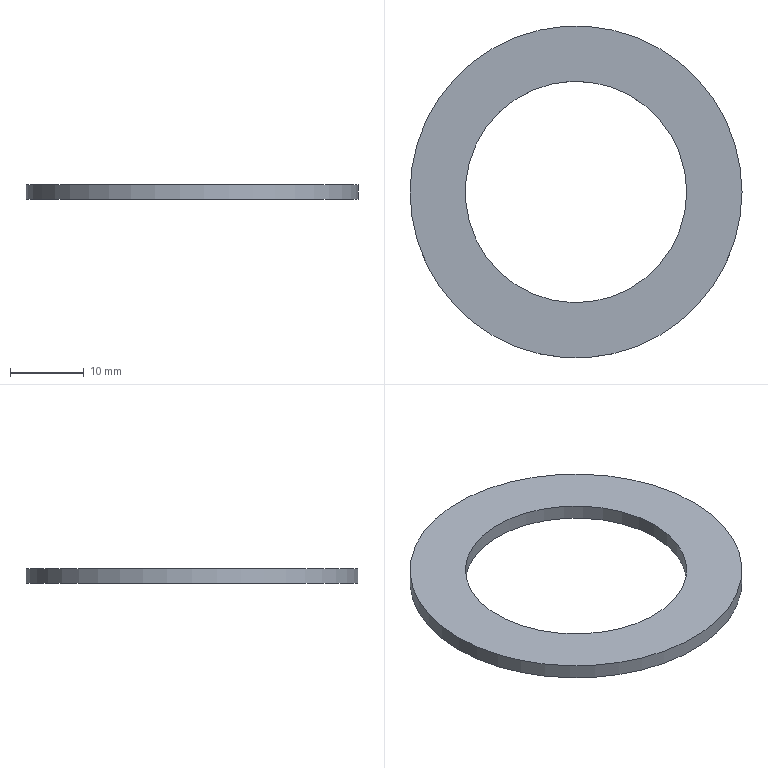Part | NX | features CYLINDER 1, DATUM_CSYS 1, HOLE PACKAGE 1, SIMPLE HOLE 1 | 1 solid | 4 faces | box 45 x 45 x 2 mm | volume 1767 mm3 | plane 2 | cylinder 2 | commonest cylinder face diameters 30 x1 45 x1
STEP:
#1=CARTESIAN_POINT('',(15.,0.,2.));
#2=VERTEX_POINT('',#1);
#3=CARTESIAN_POINT('',(0.,0.,2.));
#4=DIRECTION('',(0.,0.,1.));
#5=DIRECTION('',(1.,0.,0.));
#6=AXIS2_PLACEMENT_3D('',#3,#4,#5);
#7=CIRCLE('',#6,15.);
#8=EDGE_CURVE('',#2,#2,#7,.T.);
#9=ORIENTED_EDGE('',*,*,#8,.F.);
#10=EDGE_LOOP('',(#9));
#11=FACE_BOUND('',#10,.T.);
#12=CARTESIAN_POINT('',(-22.5,0.,2.));
#13=VERTEX_POINT('',#12);
#14=CARTESIAN_POINT('',(0.,0.,2.));
#15=DIRECTION('',(0.,0.,-1.));
#16=DIRECTION('',(-1.,0.,0.));
#17=AXIS2_PLACEMENT_3D('',#14,#15,#16);
#18=CIRCLE('',#17,22.5);
#19=EDGE_CURVE('',#13,#13,#18,.T.);
#20=ORIENTED_EDGE('',*,*,#19,.F.);
#21=EDGE_LOOP('',(#20));
#22=FACE_BOUND('',#21,.T.);
#23=CARTESIAN_POINT('',(0.,0.,2.));
#24=DIRECTION('',(0.,0.,1.));
#25=DIRECTION('',(1.,0.,0.));
#26=AXIS2_PLACEMENT_3D('',#23,#24,#25);
#27=PLANE('',#26);
#28=ADVANCED_FACE('',(#11,#22),#27,.T.);
#29=CARTESIAN_POINT('',(15.,0.,0.));
#30=VERTEX_POINT('',#29);
#31=CARTESIAN_POINT('',(0.,0.,0.));
#32=DIRECTION('',(0.,0.,1.));
#33=DIRECTION('',(1.,0.,0.));
#34=AXIS2_PLACEMENT_3D('',#31,#32,#33);
#35=CIRCLE('',#34,15.);
#36=EDGE_CURVE('',#30,#30,#35,.T.);
#37=ORIENTED_EDGE('',*,*,#36,.T.);
#38=EDGE_LOOP('',(#37));
#39=FACE_BOUND('',#38,.T.);
#40=CARTESIAN_POINT('',(22.5,0.,0.));
#41=VERTEX_POINT('',#40);
#42=CARTESIAN_POINT('',(0.,0.,0.));
#43=DIRECTION('',(0.,0.,1.));
#44=DIRECTION('',(1.,0.,0.));
#45=AXIS2_PLACEMENT_3D('',#42,#43,#44);
#46=CIRCLE('',#45,22.5);
#47=EDGE_CURVE('',#41,#41,#46,.T.);
#48=ORIENTED_EDGE('',*,*,#47,.F.);
#49=EDGE_LOOP('',(#48));
#50=FACE_BOUND('',#49,.T.);
#51=CARTESIAN_POINT('',(0.,0.,0.));
#52=DIRECTION('',(0.,0.,-1.));
#53=DIRECTION('',(-1.,0.,0.));
#54=AXIS2_PLACEMENT_3D('',#51,#52,#53);
#55=PLANE('',#54);
#56=ADVANCED_FACE('',(#39,#50),#55,.T.);
#57=ORIENTED_EDGE('',*,*,#19,.T.);
#58=EDGE_LOOP('',(#57));
#59=FACE_BOUND('',#58,.T.);
#60=ORIENTED_EDGE('',*,*,#47,.T.);
#61=EDGE_LOOP('',(#60));
#62=FACE_BOUND('',#61,.T.);
#63=CARTESIAN_POINT('',(0.,0.,0.));
#64=DIRECTION('',(0.,0.,1.));
#65=DIRECTION('',(1.,0.,0.));
#66=AXIS2_PLACEMENT_3D('',#63,#64,#65);
#67=CYLINDRICAL_SURFACE('',#66,22.5);
#68=ADVANCED_FACE('',(#59,#62),#67,.T.);
#69=ORIENTED_EDGE('',*,*,#8,.T.);
#70=EDGE_LOOP('',(#69));
#71=FACE_BOUND('',#70,.T.);
#72=ORIENTED_EDGE('',*,*,#36,.F.);
#73=EDGE_LOOP('',(#72));
#74=FACE_BOUND('',#73,.T.);
#75=CARTESIAN_POINT('',(0.,0.,0.));
#76=DIRECTION('',(0.,0.,1.));
#77=DIRECTION('',(1.,0.,0.));
#78=AXIS2_PLACEMENT_3D('',#75,#76,#77);
#79=CYLINDRICAL_SURFACE('',#78,15.);
#80=ADVANCED_FACE('',(#71,#74),#79,.F.);
#81=CLOSED_SHELL('',(#28,#56,#68,#80));
#82=MANIFOLD_SOLID_BREP('',#81);
#83=(LENGTH_UNIT()NAMED_UNIT(*)SI_UNIT(.MILLI.,.METRE.));
#84=UNCERTAINTY_MEASURE_WITH_UNIT(LENGTH_MEASURE(0.00001),#83,'','');
#85=(NAMED_UNIT(*)PLANE_ANGLE_UNIT()SI_UNIT($,.RADIAN.));
#86=(NAMED_UNIT(*)SI_UNIT($,.STERADIAN.)SOLID_ANGLE_UNIT());
#87=(GEOMETRIC_REPRESENTATION_CONTEXT(3)GLOBAL_UNCERTAINTY_ASSIGNED_CONTEXT((#84))GLOBAL_UNIT_ASSIGNED_CONTEXT((#83,#85,#86))REPRESENTATION_CONTEXT('',''));
#88=ADVANCED_BREP_SHAPE_REPRESENTATION('',(#82),#87);